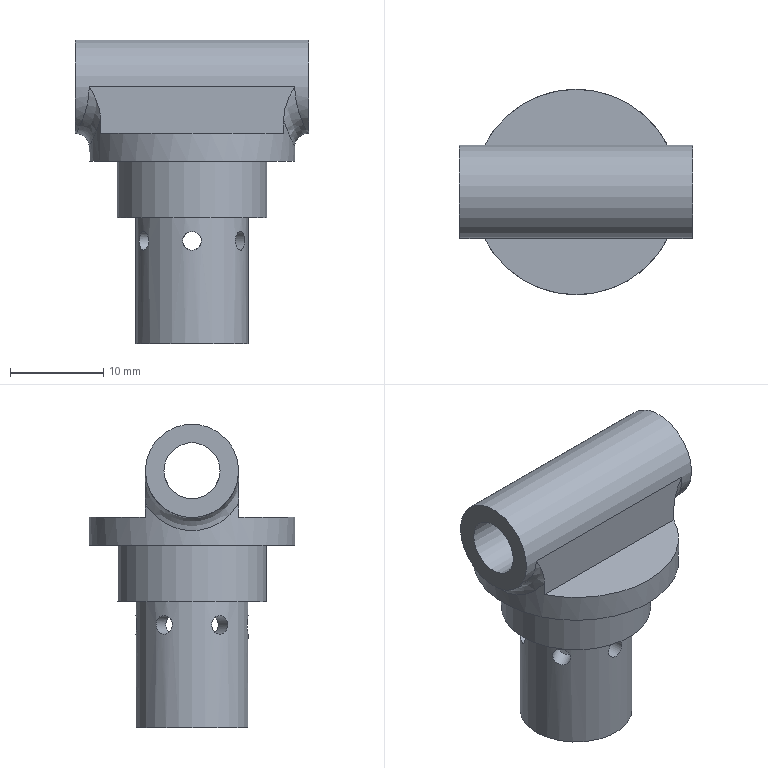Part | STEP file | 1-67.1 | 1 solid | 28 faces | box 25 x 22 x 32.5 mm | volume 4130 mm3 | cylinder 14 | plane 11 | spline 3 | commonest cylinder face diameters 2 x6 10 x2 5 x1 6 x1 8 x1 12 x1